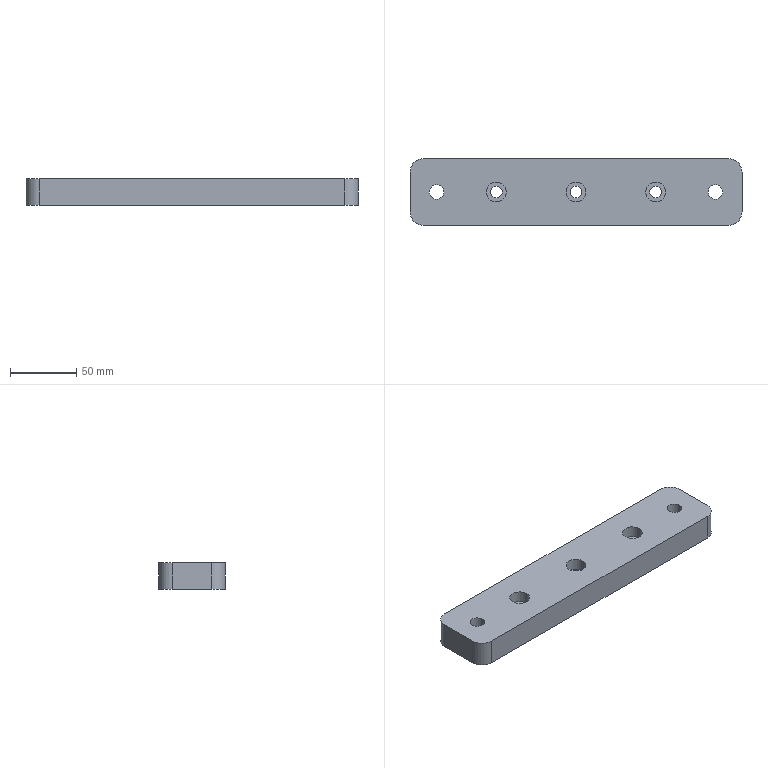Part | SolidWorks | features 3DProfileFeature 2, HoleWzd 2, Extrusion 1, Fillet 1, LPattern 1 | 1 solid | 39 faces | box 250 x 50 x 20 mm | volume 234104 mm3 | cylinder 24 | plane 11 | cone 4 | commonest cylinder face diameters 9 x6 15 x6 11 x4 18 x4 20 x4
STEP:
#1=CARTESIAN_POINT('',(64.,0.,0.025));
#2=VERTEX_POINT('',#1);
#3=CARTESIAN_POINT('',(46.,0.,0.025));
#4=VERTEX_POINT('',#3);
#5=CARTESIAN_POINT('',(55.,0.,0.025));
#6=DIRECTION('',(0.,0.,-1.));
#7=DIRECTION('',(-1.,0.,0.));
#8=AXIS2_PLACEMENT_3D('',#5,#6,#7);
#9=CIRCLE('',#8,9.);
#10=EDGE_CURVE('',#2,#4,#9,.T.);
#11=ORIENTED_EDGE('',*,*,#10,.F.);
#12=CARTESIAN_POINT('',(64.025,0.,0.));
#13=VERTEX_POINT('',#12);
#14=CARTESIAN_POINT('',(64.025,0.,0.));
#15=DIRECTION('',(0.7071,0.,-0.7071));
#16=VECTOR('',#15,1000.);
#17=LINE('',#14,#16);
#18=EDGE_CURVE('',#2,#13,#17,.T.);
#19=ORIENTED_EDGE('',*,*,#18,.T.);
#20=CARTESIAN_POINT('',(45.975,0.,0.));
#21=VERTEX_POINT('',#20);
#22=CARTESIAN_POINT('',(55.,0.,0.));
#23=DIRECTION('',(0.,0.,-1.));
#24=DIRECTION('',(-1.,0.,0.));
#25=AXIS2_PLACEMENT_3D('',#22,#23,#24);
#26=CIRCLE('',#25,9.025);
#27=EDGE_CURVE('',#13,#21,#26,.T.);
#28=ORIENTED_EDGE('',*,*,#27,.T.);
#29=CARTESIAN_POINT('',(45.975,0.,0.));
#30=DIRECTION('',(-0.7071,0.,-0.7071));
#31=VECTOR('',#30,1000.);
#32=LINE('',#29,#31);
#33=EDGE_CURVE('',#4,#21,#32,.T.);
#34=ORIENTED_EDGE('',*,*,#33,.F.);
#35=EDGE_LOOP('',(#11,#19,#28,#34));
#36=FACE_OUTER_BOUND('',#35,.T.);
#37=CARTESIAN_POINT('',(55.,0.,0.));
#38=DIRECTION('',(0.,0.,-1.));
#39=DIRECTION('',(-1.,0.,0.));
#40=AXIS2_PLACEMENT_3D('',#37,#38,#39);
#41=CONICAL_SURFACE('',#40,9.025,0.7854);
#42=ADVANCED_FACE('',(#36),#41,.F.);
#43=CARTESIAN_POINT('',(64.,0.,11.));
#44=VERTEX_POINT('',#43);
#45=CARTESIAN_POINT('',(46.,0.,11.));
#46=VERTEX_POINT('',#45);
#47=CARTESIAN_POINT('',(55.,0.,11.));
#48=DIRECTION('',(0.,0.,-1.));
#49=DIRECTION('',(-1.,0.,0.));
#50=AXIS2_PLACEMENT_3D('',#47,#48,#49);
#51=CIRCLE('',#50,9.);
#52=EDGE_CURVE('',#44,#46,#51,.T.);
#53=ORIENTED_EDGE('',*,*,#52,.F.);
#54=CARTESIAN_POINT('',(64.,0.,0.));
#55=DIRECTION('',(0.,0.,-1.));
#56=VECTOR('',#55,1000.);
#57=LINE('',#54,#56);
#58=EDGE_CURVE('',#44,#2,#57,.T.);
#59=ORIENTED_EDGE('',*,*,#58,.T.);
#60=ORIENTED_EDGE('',*,*,#10,.T.);
#61=CARTESIAN_POINT('',(46.,0.,0.));
#62=DIRECTION('',(0.,0.,-1.));
#63=VECTOR('',#62,1000.);
#64=LINE('',#61,#63);
#65=EDGE_CURVE('',#46,#4,#64,.T.);
#66=ORIENTED_EDGE('',*,*,#65,.F.);
#67=EDGE_LOOP('',(#53,#59,#60,#66));
#68=FACE_OUTER_BOUND('',#67,.T.);
#69=CARTESIAN_POINT('',(55.,0.,0.));
#70=DIRECTION('',(0.,0.,-1.));
#71=DIRECTION('',(-1.,0.,0.));
#72=AXIS2_PLACEMENT_3D('',#69,#70,#71);
#73=CYLINDRICAL_SURFACE('',#72,9.);
#74=ADVANCED_FACE('',(#68),#73,.F.);
#75=CARTESIAN_POINT('',(49.5,0.,20.));
#76=VERTEX_POINT('',#75);
#77=CARTESIAN_POINT('',(60.5,0.,20.));
#78=VERTEX_POINT('',#77);
#79=CARTESIAN_POINT('',(55.,0.,20.));
#80=DIRECTION('',(0.,0.,1.));
#81=DIRECTION('',(1.,0.,0.));
#82=AXIS2_PLACEMENT_3D('',#79,#80,#81);
#83=CIRCLE('',#82,5.5);
#84=EDGE_CURVE('',#76,#78,#83,.T.);
#85=ORIENTED_EDGE('',*,*,#84,.T.);
#86=CARTESIAN_POINT('',(60.5,0.,11.));
#87=VERTEX_POINT('',#86);
#88=CARTESIAN_POINT('',(60.5,0.,0.));
#89=DIRECTION('',(0.,0.,-1.));
#90=VECTOR('',#89,1000.);
#91=LINE('',#88,#90);
#92=EDGE_CURVE('',#78,#87,#91,.T.);
#93=ORIENTED_EDGE('',*,*,#92,.T.);
#94=CARTESIAN_POINT('',(49.5,0.,11.));
#95=VERTEX_POINT('',#94);
#96=CARTESIAN_POINT('',(55.,0.,11.));
#97=DIRECTION('',(0.,0.,-1.));
#98=DIRECTION('',(-1.,0.,0.));
#99=AXIS2_PLACEMENT_3D('',#96,#97,#98);
#100=CIRCLE('',#99,5.5);
#101=EDGE_CURVE('',#87,#95,#100,.T.);
#102=ORIENTED_EDGE('',*,*,#101,.T.);
#103=CARTESIAN_POINT('',(49.5,0.,0.));
#104=DIRECTION('',(0.,0.,-1.));
#105=VECTOR('',#104,1000.);
#106=LINE('',#103,#105);
#107=EDGE_CURVE('',#76,#95,#106,.T.);
#108=ORIENTED_EDGE('',*,*,#107,.F.);
#109=EDGE_LOOP('',(#85,#93,#102,#108));
#110=FACE_OUTER_BOUND('',#109,.T.);
#111=CARTESIAN_POINT('',(55.,0.,0.));
#112=DIRECTION('',(0.,0.,-1.));
#113=DIRECTION('',(-1.,0.,0.));
#114=AXIS2_PLACEMENT_3D('',#111,#112,#113);
#115=CYLINDRICAL_SURFACE('',#114,5.5);
#116=ADVANCED_FACE('',(#110),#115,.F.);
#117=CARTESIAN_POINT('',(-146.,0.,0.025));
#118=VERTEX_POINT('',#117);
#119=CARTESIAN_POINT('',(-164.,0.,0.025));
#120=VERTEX_POINT('',#119);
#121=CARTESIAN_POINT('',(-155.,0.,0.025));
#122=DIRECTION('',(0.,0.,-1.));
#123=DIRECTION('',(-1.,0.,0.));
#124=AXIS2_PLACEMENT_3D('',#121,#122,#123);
#125=CIRCLE('',#124,9.);
#126=EDGE_CURVE('',#118,#120,#125,.T.);
#127=ORIENTED_EDGE('',*,*,#126,.F.);
#128=CARTESIAN_POINT('',(-145.975,0.,0.));
#129=VERTEX_POINT('',#128);
#130=CARTESIAN_POINT('',(-145.975,0.,0.));
#131=DIRECTION('',(0.7071,0.,-0.7071));
#132=VECTOR('',#131,1000.);
#133=LINE('',#130,#132);
#134=EDGE_CURVE('',#118,#129,#133,.T.);
#135=ORIENTED_EDGE('',*,*,#134,.T.);
#136=CARTESIAN_POINT('',(-164.025,0.,0.));
#137=VERTEX_POINT('',#136);
#138=CARTESIAN_POINT('',(-155.,0.,0.));
#139=DIRECTION('',(0.,0.,-1.));
#140=DIRECTION('',(-1.,0.,0.));
#141=AXIS2_PLACEMENT_3D('',#138,#139,#140);
#142=CIRCLE('',#141,9.025);
#143=EDGE_CURVE('',#129,#137,#142,.T.);
#144=ORIENTED_EDGE('',*,*,#143,.T.);
#145=CARTESIAN_POINT('',(-164.025,0.,0.));
#146=DIRECTION('',(-0.7071,0.,-0.7071));
#147=VECTOR('',#146,1000.);
#148=LINE('',#145,#147);
#149=EDGE_CURVE('',#120,#137,#148,.T.);
#150=ORIENTED_EDGE('',*,*,#149,.F.);
#151=EDGE_LOOP('',(#127,#135,#144,#150));
#152=FACE_OUTER_BOUND('',#151,.T.);
#153=CARTESIAN_POINT('',(-155.,0.,0.));
#154=DIRECTION('',(0.,0.,-1.));
#155=DIRECTION('',(-1.,0.,0.));
#156=AXIS2_PLACEMENT_3D('',#153,#154,#155);
#157=CONICAL_SURFACE('',#156,9.025,0.7854);
#158=ADVANCED_FACE('',(#152),#157,.F.);
#159=CARTESIAN_POINT('',(-146.,0.,11.));
#160=VERTEX_POINT('',#159);
#161=CARTESIAN_POINT('',(-164.,0.,11.));
#162=VERTEX_POINT('',#161);
#163=CARTESIAN_POINT('',(-155.,0.,11.));
#164=DIRECTION('',(0.,0.,-1.));
#165=DIRECTION('',(-1.,0.,0.));
#166=AXIS2_PLACEMENT_3D('',#163,#164,#165);
#167=CIRCLE('',#166,9.);
#168=EDGE_CURVE('',#160,#162,#167,.T.);
#169=ORIENTED_EDGE('',*,*,#168,.F.);
#170=CARTESIAN_POINT('',(-146.,0.,0.));
#171=DIRECTION('',(0.,0.,-1.));
#172=VECTOR('',#171,1000.);
#173=LINE('',#170,#172);
#174=EDGE_CURVE('',#160,#118,#173,.T.);
#175=ORIENTED_EDGE('',*,*,#174,.T.);
#176=ORIENTED_EDGE('',*,*,#126,.T.);
#177=CARTESIAN_POINT('',(-164.,0.,0.));
#178=DIRECTION('',(0.,0.,-1.));
#179=VECTOR('',#178,1000.);
#180=LINE('',#177,#179);
#181=EDGE_CURVE('',#162,#120,#180,.T.);
#182=ORIENTED_EDGE('',*,*,#181,.F.);
#183=EDGE_LOOP('',(#169,#175,#176,#182));
#184=FACE_OUTER_BOUND('',#183,.T.);
#185=CARTESIAN_POINT('',(-155.,0.,0.));
#186=DIRECTION('',(0.,0.,-1.));
#187=DIRECTION('',(-1.,0.,0.));
#188=AXIS2_PLACEMENT_3D('',#185,#186,#187);
#189=CYLINDRICAL_SURFACE('',#188,9.);
#190=ADVANCED_FACE('',(#184),#189,.F.);
#191=CARTESIAN_POINT('',(-160.5,0.,20.));
#192=VERTEX_POINT('',#191);
#193=CARTESIAN_POINT('',(-149.5,0.,20.));
#194=VERTEX_POINT('',#193);
#195=CARTESIAN_POINT('',(-155.,0.,20.));
#196=DIRECTION('',(0.,0.,1.));
#197=DIRECTION('',(1.,0.,0.));
#198=AXIS2_PLACEMENT_3D('',#195,#196,#197);
#199=CIRCLE('',#198,5.5);
#200=EDGE_CURVE('',#192,#194,#199,.T.);
#201=ORIENTED_EDGE('',*,*,#200,.T.);
#202=CARTESIAN_POINT('',(-149.5,0.,11.));
#203=VERTEX_POINT('',#202);
#204=CARTESIAN_POINT('',(-149.5,0.,0.));
#205=DIRECTION('',(0.,0.,-1.));
#206=VECTOR('',#205,1000.);
#207=LINE('',#204,#206);
#208=EDGE_CURVE('',#194,#203,#207,.T.);
#209=ORIENTED_EDGE('',*,*,#208,.T.);
#210=CARTESIAN_POINT('',(-160.5,0.,11.));
#211=VERTEX_POINT('',#210);
#212=CARTESIAN_POINT('',(-155.,0.,11.));
#213=DIRECTION('',(0.,0.,-1.));
#214=DIRECTION('',(-1.,0.,0.));
#215=AXIS2_PLACEMENT_3D('',#212,#213,#214);
#216=CIRCLE('',#215,5.5);
#217=EDGE_CURVE('',#203,#211,#216,.T.);
#218=ORIENTED_EDGE('',*,*,#217,.T.);
#219=CARTESIAN_POINT('',(-160.5,0.,0.));
#220=DIRECTION('',(0.,0.,-1.));
#221=VECTOR('',#220,1000.);
#222=LINE('',#219,#221);
#223=EDGE_CURVE('',#192,#211,#222,.T.);
#224=ORIENTED_EDGE('',*,*,#223,.F.);
#225=EDGE_LOOP('',(#201,#209,#218,#224));
#226=FACE_OUTER_BOUND('',#225,.T.);
#227=CARTESIAN_POINT('',(-155.,0.,0.));
#228=DIRECTION('',(0.,0.,-1.));
#229=DIRECTION('',(-1.,0.,0.));
#230=AXIS2_PLACEMENT_3D('',#227,#228,#229);
#231=CYLINDRICAL_SURFACE('',#230,5.5);
#232=ADVANCED_FACE('',(#226),#231,.F.);
#233=CARTESIAN_POINT('',(-117.5,0.,11.));
#234=VERTEX_POINT('',#233);
#235=CARTESIAN_POINT('',(-102.5,0.,11.));
#236=VERTEX_POINT('',#235);
#237=CARTESIAN_POINT('',(-110.,0.,11.));
#238=DIRECTION('',(0.,0.,1.));
#239=DIRECTION('',(1.,0.,0.));
#240=AXIS2_PLACEMENT_3D('',#237,#238,#239);
#241=CIRCLE('',#240,7.5);
#242=EDGE_CURVE('',#234,#236,#241,.T.);
#243=ORIENTED_EDGE('',*,*,#242,.F.);
#244=CARTESIAN_POINT('',(-117.5,0.,20.));
#245=VERTEX_POINT('',#244);
#246=CARTESIAN_POINT('',(-117.5,0.,20.));
#247=DIRECTION('',(0.,0.,1.));
#248=VECTOR('',#247,1000.);
#249=LINE('',#246,#248);
#250=EDGE_CURVE('',#234,#245,#249,.T.);
#251=ORIENTED_EDGE('',*,*,#250,.T.);
#252=CARTESIAN_POINT('',(-102.5,0.,20.));
#253=VERTEX_POINT('',#252);
#254=CARTESIAN_POINT('',(-110.,0.,20.));
#255=DIRECTION('',(0.,0.,1.));
#256=DIRECTION('',(1.,0.,0.));
#257=AXIS2_PLACEMENT_3D('',#254,#255,#256);
#258=CIRCLE('',#257,7.5);
#259=EDGE_CURVE('',#245,#253,#258,.T.);
#260=ORIENTED_EDGE('',*,*,#259,.T.);
#261=CARTESIAN_POINT('',(-102.5,0.,20.));
#262=DIRECTION('',(0.,0.,1.));
#263=VECTOR('',#262,1000.);
#264=LINE('',#261,#263);
#265=EDGE_CURVE('',#236,#253,#264,.T.);
#266=ORIENTED_EDGE('',*,*,#265,.F.);
#267=EDGE_LOOP('',(#243,#251,#260,#266));
#268=FACE_OUTER_BOUND('',#267,.T.);
#269=CARTESIAN_POINT('',(-110.,0.,20.));
#270=DIRECTION('',(0.,0.,1.));
#271=DIRECTION('',(1.,0.,0.));
#272=AXIS2_PLACEMENT_3D('',#269,#270,#271);
#273=CYLINDRICAL_SURFACE('',#272,7.5);
#274=ADVANCED_FACE('',(#268),#273,.F.);
#275=CARTESIAN_POINT('',(-114.5,0.,0.));
#276=VERTEX_POINT('',#275);
#277=CARTESIAN_POINT('',(-105.5,0.,0.));
#278=VERTEX_POINT('',#277);
#279=CARTESIAN_POINT('',(-110.,0.,0.));
#280=DIRECTION('',(0.,0.,1.));
#281=DIRECTION('',(1.,0.,0.));
#282=AXIS2_PLACEMENT_3D('',#279,#280,#281);
#283=CIRCLE('',#282,4.5);
#284=EDGE_CURVE('',#276,#278,#283,.T.);
#285=ORIENTED_EDGE('',*,*,#284,.F.);
#286=CARTESIAN_POINT('',(-114.5,0.,11.));
#287=VERTEX_POINT('',#286);
#288=CARTESIAN_POINT('',(-114.5,0.,20.));
#289=DIRECTION('',(0.,0.,1.));
#290=VECTOR('',#289,1000.);
#291=LINE('',#288,#290);
#292=EDGE_CURVE('',#276,#287,#291,.T.);
#293=ORIENTED_EDGE('',*,*,#292,.T.);
#294=CARTESIAN_POINT('',(-105.5,0.,11.));
#295=VERTEX_POINT('',#294);
#296=CARTESIAN_POINT('',(-110.,0.,11.));
#297=DIRECTION('',(0.,0.,1.));
#298=DIRECTION('',(1.,0.,0.));
#299=AXIS2_PLACEMENT_3D('',#296,#297,#298);
#300=CIRCLE('',#299,4.5);
#301=EDGE_CURVE('',#287,#295,#300,.T.);
#302=ORIENTED_EDGE('',*,*,#301,.T.);
#303=CARTESIAN_POINT('',(-105.5,0.,20.));
#304=DIRECTION('',(0.,0.,1.));
#305=VECTOR('',#304,1000.);
#306=LINE('',#303,#305);
#307=EDGE_CURVE('',#278,#295,#306,.T.);
#308=ORIENTED_EDGE('',*,*,#307,.F.);
#309=EDGE_LOOP('',(#285,#293,#302,#308));
#310=FACE_OUTER_BOUND('',#309,.T.);
#311=CARTESIAN_POINT('',(-110.,0.,20.));
#312=DIRECTION('',(0.,0.,1.));
#313=DIRECTION('',(1.,0.,0.));
#314=AXIS2_PLACEMENT_3D('',#311,#312,#313);
#315=CYLINDRICAL_SURFACE('',#314,4.5);
#316=ADVANCED_FACE('',(#310),#315,.F.);
#317=CARTESIAN_POINT('',(-57.5,0.,11.));
#318=VERTEX_POINT('',#317);
#319=CARTESIAN_POINT('',(-42.5,0.,11.));
#320=VERTEX_POINT('',#319);
#321=CARTESIAN_POINT('',(-50.,0.,11.));
#322=DIRECTION('',(0.,0.,1.));
#323=DIRECTION('',(1.,0.,0.));
#324=AXIS2_PLACEMENT_3D('',#321,#322,#323);
#325=CIRCLE('',#324,7.5);
#326=EDGE_CURVE('',#318,#320,#325,.T.);
#327=ORIENTED_EDGE('',*,*,#326,.F.);
#328=CARTESIAN_POINT('',(-57.5,0.,20.));
#329=VERTEX_POINT('',#328);
#330=CARTESIAN_POINT('',(-57.5,0.,20.));
#331=DIRECTION('',(0.,0.,1.));
#332=VECTOR('',#331,1000.);
#333=LINE('',#330,#332);
#334=EDGE_CURVE('',#318,#329,#333,.T.);
#335=ORIENTED_EDGE('',*,*,#334,.T.);
#336=CARTESIAN_POINT('',(-42.5,0.,20.));
#337=VERTEX_POINT('',#336);
#338=CARTESIAN_POINT('',(-50.,0.,20.));
#339=DIRECTION('',(0.,0.,1.));
#340=DIRECTION('',(1.,0.,0.));
#341=AXIS2_PLACEMENT_3D('',#338,#339,#340);
#342=CIRCLE('',#341,7.5);
#343=EDGE_CURVE('',#329,#337,#342,.T.);
#344=ORIENTED_EDGE('',*,*,#343,.T.);
#345=CARTESIAN_POINT('',(-42.5,0.,20.));
#346=DIRECTION('',(0.,0.,1.));
#347=VECTOR('',#346,1000.);
#348=LINE('',#345,#347);
#349=EDGE_CURVE('',#320,#337,#348,.T.);
#350=ORIENTED_EDGE('',*,*,#349,.F.);
#351=EDGE_LOOP('',(#327,#335,#344,#350));
#352=FACE_OUTER_BOUND('',#351,.T.);
#353=CARTESIAN_POINT('',(-50.,0.,20.));
#354=DIRECTION('',(0.,0.,1.));
#355=DIRECTION('',(1.,0.,0.));
#356=AXIS2_PLACEMENT_3D('',#353,#354,#355);
#357=CYLINDRICAL_SURFACE('',#356,7.5);
#358=ADVANCED_FACE('',(#352),#357,.F.);
#359=CARTESIAN_POINT('',(-54.5,0.,0.));
#360=VERTEX_POINT('',#359);
#361=CARTESIAN_POINT('',(-45.5,0.,0.));
#362=VERTEX_POINT('',#361);
#363=CARTESIAN_POINT('',(-50.,0.,0.));
#364=DIRECTION('',(0.,0.,1.));
#365=DIRECTION('',(1.,0.,0.));
#366=AXIS2_PLACEMENT_3D('',#363,#364,#365);
#367=CIRCLE('',#366,4.5);
#368=EDGE_CURVE('',#360,#362,#367,.T.);
#369=ORIENTED_EDGE('',*,*,#368,.F.);
#370=CARTESIAN_POINT('',(-54.5,0.,11.));
#371=VERTEX_POINT('',#370);
#372=CARTESIAN_POINT('',(-54.5,0.,20.));
#373=DIRECTION('',(0.,0.,1.));
#374=VECTOR('',#373,1000.);
#375=LINE('',#372,#374);
#376=EDGE_CURVE('',#360,#371,#375,.T.);
#377=ORIENTED_EDGE('',*,*,#376,.T.);
#378=CARTESIAN_POINT('',(-45.5,0.,11.));
#379=VERTEX_POINT('',#378);
#380=CARTESIAN_POINT('',(-50.,0.,11.));
#381=DIRECTION('',(0.,0.,1.));
#382=DIRECTION('',(1.,0.,0.));
#383=AXIS2_PLACEMENT_3D('',#380,#381,#382);
#384=CIRCLE('',#383,4.5);
#385=EDGE_CURVE('',#371,#379,#384,.T.);
#386=ORIENTED_EDGE('',*,*,#385,.T.);
#387=CARTESIAN_POINT('',(-45.5,0.,20.));
#388=DIRECTION('',(0.,0.,1.));
#389=VECTOR('',#388,1000.);
#390=LINE('',#387,#389);
#391=EDGE_CURVE('',#362,#379,#390,.T.);
#392=ORIENTED_EDGE('',*,*,#391,.F.);
#393=EDGE_LOOP('',(#369,#377,#386,#392));
#394=FACE_OUTER_BOUND('',#393,.T.);
#395=CARTESIAN_POINT('',(-50.,0.,20.));
#396=DIRECTION('',(0.,0.,1.));
#397=DIRECTION('',(1.,0.,0.));
#398=AXIS2_PLACEMENT_3D('',#395,#396,#397);
#399=CYLINDRICAL_SURFACE('',#398,4.5);
#400=ADVANCED_FACE('',(#394),#399,.F.);
#401=CARTESIAN_POINT('',(2.5,0.,11.));
#402=VERTEX_POINT('',#401);
#403=CARTESIAN_POINT('',(17.5,0.,11.));
#404=VERTEX_POINT('',#403);
#405=CARTESIAN_POINT('',(10.,0.,11.));
#406=DIRECTION('',(0.,0.,1.));
#407=DIRECTION('',(1.,0.,0.));
#408=AXIS2_PLACEMENT_3D('',#405,#406,#407);
#409=CIRCLE('',#408,7.5);
#410=EDGE_CURVE('',#402,#404,#409,.T.);
#411=ORIENTED_EDGE('',*,*,#410,.F.);
#412=CARTESIAN_POINT('',(2.5,0.,20.));
#413=VERTEX_POINT('',#412);
#414=CARTESIAN_POINT('',(2.5,0.,20.));
#415=DIRECTION('',(0.,0.,1.));
#416=VECTOR('',#415,1000.);
#417=LINE('',#414,#416);
#418=EDGE_CURVE('',#402,#413,#417,.T.);
#419=ORIENTED_EDGE('',*,*,#418,.T.);
#420=CARTESIAN_POINT('',(17.5,0.,20.));
#421=VERTEX_POINT('',#420);
#422=CARTESIAN_POINT('',(10.,0.,20.));
#423=DIRECTION('',(0.,0.,1.));
#424=DIRECTION('',(1.,0.,0.));
#425=AXIS2_PLACEMENT_3D('',#422,#423,#424);
#426=CIRCLE('',#425,7.5);
#427=EDGE_CURVE('',#413,#421,#426,.T.);
#428=ORIENTED_EDGE('',*,*,#427,.T.);
#429=CARTESIAN_POINT('',(17.5,0.,20.));
#430=DIRECTION('',(0.,0.,1.));
#431=VECTOR('',#430,1000.);
#432=LINE('',#429,#431);
#433=EDGE_CURVE('',#404,#421,#432,.T.);
#434=ORIENTED_EDGE('',*,*,#433,.F.);
#435=EDGE_LOOP('',(#411,#419,#428,#434));
#436=FACE_OUTER_BOUND('',#435,.T.);
#437=CARTESIAN_POINT('',(10.,0.,20.));
#438=DIRECTION('',(0.,0.,1.));
#439=DIRECTION('',(1.,0.,0.));
#440=AXIS2_PLACEMENT_3D('',#437,#438,#439);
#441=CYLINDRICAL_SURFACE('',#440,7.5);
#442=ADVANCED_FACE('',(#436),#441,.F.);
#443=CARTESIAN_POINT('',(5.5,0.,0.));
#444=VERTEX_POINT('',#443);
#445=CARTESIAN_POINT('',(14.5,0.,0.));
#446=VERTEX_POINT('',#445);
#447=CARTESIAN_POINT('',(10.,0.,0.));
#448=DIRECTION('',(0.,0.,1.));
#449=DIRECTION('',(1.,0.,0.));
#450=AXIS2_PLACEMENT_3D('',#447,#448,#449);
#451=CIRCLE('',#450,4.5);
#452=EDGE_CURVE('',#444,#446,#451,.T.);
#453=ORIENTED_EDGE('',*,*,#452,.F.);
#454=CARTESIAN_POINT('',(5.5,0.,11.));
#455=VERTEX_POINT('',#454);
#456=CARTESIAN_POINT('',(5.5,0.,20.));
#457=DIRECTION('',(0.,0.,1.));
#458=VECTOR('',#457,1000.);
#459=LINE('',#456,#458);
#460=EDGE_CURVE('',#444,#455,#459,.T.);
#461=ORIENTED_EDGE('',*,*,#460,.T.);
#462=CARTESIAN_POINT('',(14.5,0.,11.));
#463=VERTEX_POINT('',#462);
#464=CARTESIAN_POINT('',(10.,0.,11.));
#465=DIRECTION('',(0.,0.,1.));
#466=DIRECTION('',(1.,0.,0.));
#467=AXIS2_PLACEMENT_3D('',#464,#465,#466);
#468=CIRCLE('',#467,4.5);
#469=EDGE_CURVE('',#455,#463,#468,.T.);
#470=ORIENTED_EDGE('',*,*,#469,.T.);
#471=CARTESIAN_POINT('',(14.5,0.,20.));
#472=DIRECTION('',(0.,0.,1.));
#473=VECTOR('',#472,1000.);
#474=LINE('',#471,#473);
#475=EDGE_CURVE('',#446,#463,#474,.T.);
#476=ORIENTED_EDGE('',*,*,#475,.F.);
#477=EDGE_LOOP('',(#453,#461,#470,#476));
#478=FACE_OUTER_BOUND('',#477,.T.);
#479=CARTESIAN_POINT('',(10.,0.,20.));
#480=DIRECTION('',(0.,0.,1.));
#481=DIRECTION('',(1.,0.,0.));
#482=AXIS2_PLACEMENT_3D('',#479,#480,#481);
#483=CYLINDRICAL_SURFACE('',#482,4.5);
#484=ADVANCED_FACE('',(#478),#483,.F.);
#485=CARTESIAN_POINT('',(-175.,15.,0.));
#486=VERTEX_POINT('',#485);
#487=CARTESIAN_POINT('',(-175.,-15.,0.));
#488=VERTEX_POINT('',#487);
#489=CARTESIAN_POINT('',(-175.,-25.,0.));
#490=DIRECTION('',(0.,-1.,0.));
#491=VECTOR('',#490,1000.);
#492=LINE('',#489,#491);
#493=EDGE_CURVE('',#486,#488,#492,.T.);
#494=ORIENTED_EDGE('',*,*,#493,.T.);
#495=CARTESIAN_POINT('',(-175.,-15.,20.));
#496=VERTEX_POINT('',#495);
#497=CARTESIAN_POINT('',(-175.,-15.,20.));
#498=DIRECTION('',(0.,0.,1.));
#499=VECTOR('',#498,1000.);
#500=LINE('',#497,#499);
#501=EDGE_CURVE('',#488,#496,#500,.T.);
#502=ORIENTED_EDGE('',*,*,#501,.T.);
#503=CARTESIAN_POINT('',(-175.,15.,20.));
#504=VERTEX_POINT('',#503);
#505=CARTESIAN_POINT('',(-175.,-25.,20.));
#506=DIRECTION('',(0.,-1.,0.));
#507=VECTOR('',#506,1000.);
#508=LINE('',#505,#507);
#509=EDGE_CURVE('',#504,#496,#508,.T.);
#510=ORIENTED_EDGE('',*,*,#509,.F.);
#511=CARTESIAN_POINT('',(-175.,15.,20.));
#512=DIRECTION('',(0.,0.,-1.));
#513=VECTOR('',#512,1000.);
#514=LINE('',#511,#513);
#515=EDGE_CURVE('',#504,#486,#514,.T.);
#516=ORIENTED_EDGE('',*,*,#515,.T.);
#517=EDGE_LOOP('',(#494,#502,#510,#516));
#518=FACE_OUTER_BOUND('',#517,.T.);
#519=CARTESIAN_POINT('',(-175.,-25.,20.));
#520=DIRECTION('',(1.,0.,0.));
#521=DIRECTION('',(0.,0.,-1.));
#522=AXIS2_PLACEMENT_3D('',#519,#520,#521);
#523=PLANE('',#522);
#524=ADVANCED_FACE('',(#518),#523,.F.);
#525=CARTESIAN_POINT('',(-165.,-25.,0.));
#526=VERTEX_POINT('',#525);
#527=CARTESIAN_POINT('',(65.,-25.,0.));
#528=VERTEX_POINT('',#527);
#529=CARTESIAN_POINT('',(75.,-25.,0.));
#530=DIRECTION('',(1.,0.,0.));
#531=VECTOR('',#530,1000.);
#532=LINE('',#529,#531);
#533=EDGE_CURVE('',#526,#528,#532,.T.);
#534=ORIENTED_EDGE('',*,*,#533,.T.);
#535=CARTESIAN_POINT('',(65.,-25.,20.));
#536=VERTEX_POINT('',#535);
#537=CARTESIAN_POINT('',(65.,-25.,20.));
#538=DIRECTION('',(0.,0.,1.));
#539=VECTOR('',#538,1000.);
#540=LINE('',#537,#539);
#541=EDGE_CURVE('',#528,#536,#540,.T.);
#542=ORIENTED_EDGE('',*,*,#541,.T.);
#543=CARTESIAN_POINT('',(-165.,-25.,20.));
#544=VERTEX_POINT('',#543);
#545=CARTESIAN_POINT('',(75.,-25.,20.));
#546=DIRECTION('',(1.,0.,0.));
#547=VECTOR('',#546,1000.);
#548=LINE('',#545,#547);
#549=EDGE_CURVE('',#544,#536,#548,.T.);
#550=ORIENTED_EDGE('',*,*,#549,.F.);
#551=CARTESIAN_POINT('',(-165.,-25.,20.));
#552=DIRECTION('',(0.,0.,-1.));
#553=VECTOR('',#552,1000.);
#554=LINE('',#551,#553);
#555=EDGE_CURVE('',#544,#526,#554,.T.);
#556=ORIENTED_EDGE('',*,*,#555,.T.);
#557=EDGE_LOOP('',(#534,#542,#550,#556));
#558=FACE_OUTER_BOUND('',#557,.T.);
#559=CARTESIAN_POINT('',(75.,-25.,20.));
#560=DIRECTION('',(0.,1.,0.));
#561=DIRECTION('',(-1.,0.,0.));
#562=AXIS2_PLACEMENT_3D('',#559,#560,#561);
#563=PLANE('',#562);
#564=ADVANCED_FACE('',(#558),#563,.F.);
#565=CARTESIAN_POINT('',(75.,-15.,20.));
#566=VERTEX_POINT('',#565);
#567=CARTESIAN_POINT('',(75.,15.,20.));
#568=VERTEX_POINT('',#567);
#569=CARTESIAN_POINT('',(75.,-25.,20.));
#570=DIRECTION('',(0.,1.,0.));
#571=VECTOR('',#570,1000.);
#572=LINE('',#569,#571);
#573=EDGE_CURVE('',#566,#568,#572,.T.);
#574=ORIENTED_EDGE('',*,*,#573,.F.);
#575=CARTESIAN_POINT('',(75.,-15.,0.));
#576=VERTEX_POINT('',#575);
#577=CARTESIAN_POINT('',(75.,-15.,20.));
#578=DIRECTION('',(0.,0.,-1.));
#579=VECTOR('',#578,1000.);
#580=LINE('',#577,#579);
#581=EDGE_CURVE('',#566,#576,#580,.T.);
#582=ORIENTED_EDGE('',*,*,#581,.T.);
#583=CARTESIAN_POINT('',(75.,15.,0.));
#584=VERTEX_POINT('',#583);
#585=CARTESIAN_POINT('',(75.,-25.,0.));
#586=DIRECTION('',(0.,1.,0.));
#587=VECTOR('',#586,1000.);
#588=LINE('',#585,#587);
#589=EDGE_CURVE('',#576,#584,#588,.T.);
#590=ORIENTED_EDGE('',*,*,#589,.T.);
#591=CARTESIAN_POINT('',(75.,15.,20.));
#592=DIRECTION('',(0.,0.,1.));
#593=VECTOR('',#592,1000.);
#594=LINE('',#591,#593);
#595=EDGE_CURVE('',#584,#568,#594,.T.);
#596=ORIENTED_EDGE('',*,*,#595,.T.);
#597=EDGE_LOOP('',(#574,#582,#590,#596));
#598=FACE_OUTER_BOUND('',#597,.T.);
#599=CARTESIAN_POINT('',(75.,-25.,20.));
#600=DIRECTION('',(-1.,0.,0.));
#601=DIRECTION('',(0.,0.,1.));
#602=AXIS2_PLACEMENT_3D('',#599,#600,#601);
#603=PLANE('',#602);
#604=ADVANCED_FACE('',(#598),#603,.F.);
#605=CARTESIAN_POINT('',(65.,25.,0.));
#606=VERTEX_POINT('',#605);
#607=CARTESIAN_POINT('',(-165.,25.,0.));
#608=VERTEX_POINT('',#607);
#609=CARTESIAN_POINT('',(75.,25.,0.));
#610=DIRECTION('',(-1.,0.,0.));
#611=VECTOR('',#610,1000.);
#612=LINE('',#609,#611);
#613=EDGE_CURVE('',#606,#608,#612,.T.);
#614=ORIENTED_EDGE('',*,*,#613,.T.);
#615=CARTESIAN_POINT('',(-165.,25.,20.));
#616=VERTEX_POINT('',#615);
#617=CARTESIAN_POINT('',(-165.,25.,20.));
#618=DIRECTION('',(0.,0.,1.));
#619=VECTOR('',#618,1000.);
#620=LINE('',#617,#619);
#621=EDGE_CURVE('',#608,#616,#620,.T.);
#622=ORIENTED_EDGE('',*,*,#621,.T.);
#623=CARTESIAN_POINT('',(65.,25.,20.));
#624=VERTEX_POINT('',#623);
#625=CARTESIAN_POINT('',(75.,25.,20.));
#626=DIRECTION('',(-1.,0.,0.));
#627=VECTOR('',#626,1000.);
#628=LINE('',#625,#627);
#629=EDGE_CURVE('',#624,#616,#628,.T.);
#630=ORIENTED_EDGE('',*,*,#629,.F.);
#631=CARTESIAN_POINT('',(65.,25.,20.));
#632=DIRECTION('',(0.,0.,-1.));
#633=VECTOR('',#632,1000.);
#634=LINE('',#631,#633);
#635=EDGE_CURVE('',#624,#606,#634,.T.);
#636=ORIENTED_EDGE('',*,*,#635,.T.);
#637=EDGE_LOOP('',(#614,#622,#630,#636));
#638=FACE_OUTER_BOUND('',#637,.T.);
#639=CARTESIAN_POINT('',(75.,25.,20.));
#640=DIRECTION('',(0.,-1.,0.));
#641=DIRECTION('',(1.,0.,0.));
#642=AXIS2_PLACEMENT_3D('',#639,#640,#641);
#643=PLANE('',#642);
#644=ADVANCED_FACE('',(#638),#643,.F.);
#645=ORIENTED_EDGE('',*,*,#84,.F.);
#646=CARTESIAN_POINT('',(55.,0.,20.));
#647=DIRECTION('',(0.,0.,1.));
#648=DIRECTION('',(1.,0.,0.));
#649=AXIS2_PLACEMENT_3D('',#646,#647,#648);
#650=CIRCLE('',#649,5.5);
#651=EDGE_CURVE('',#78,#76,#650,.T.);
#652=ORIENTED_EDGE('',*,*,#651,.F.);
#653=EDGE_LOOP('',(#645,#652));
#654=FACE_BOUND('',#653,.T.);
#655=ORIENTED_EDGE('',*,*,#200,.F.);
#656=CARTESIAN_POINT('',(-155.,0.,20.));
#657=DIRECTION('',(0.,0.,1.));
#658=DIRECTION('',(1.,0.,0.));
#659=AXIS2_PLACEMENT_3D('',#656,#657,#658);
#660=CIRCLE('',#659,5.5);
#661=EDGE_CURVE('',#194,#192,#660,.T.);
#662=ORIENTED_EDGE('',*,*,#661,.F.);
#663=EDGE_LOOP('',(#655,#662));
#664=FACE_BOUND('',#663,.T.);
#665=CARTESIAN_POINT('',(-110.,0.,20.));
#666=DIRECTION('',(0.,0.,1.));
#667=DIRECTION('',(1.,0.,0.));
#668=AXIS2_PLACEMENT_3D('',#665,#666,#667);
#669=CIRCLE('',#668,7.5);
#670=EDGE_CURVE('',#253,#245,#669,.T.);
#671=ORIENTED_EDGE('',*,*,#670,.F.);
#672=ORIENTED_EDGE('',*,*,#259,.F.);
#673=EDGE_LOOP('',(#671,#672));
#674=FACE_BOUND('',#673,.T.);
#675=CARTESIAN_POINT('',(-50.,0.,20.));
#676=DIRECTION('',(0.,0.,1.));
#677=DIRECTION('',(1.,0.,0.));
#678=AXIS2_PLACEMENT_3D('',#675,#676,#677);
#679=CIRCLE('',#678,7.5);
#680=EDGE_CURVE('',#337,#329,#679,.T.);
#681=ORIENTED_EDGE('',*,*,#680,.F.);
#682=ORIENTED_EDGE('',*,*,#343,.F.);
#683=EDGE_LOOP('',(#681,#682));
#684=FACE_BOUND('',#683,.T.);
#685=CARTESIAN_POINT('',(10.,0.,20.));
#686=DIRECTION('',(0.,0.,1.));
#687=DIRECTION('',(1.,0.,0.));
#688=AXIS2_PLACEMENT_3D('',#685,#686,#687);
#689=CIRCLE('',#688,7.5);
#690=EDGE_CURVE('',#421,#413,#689,.T.);
#691=ORIENTED_EDGE('',*,*,#690,.F.);
#692=ORIENTED_EDGE('',*,*,#427,.F.);
#693=EDGE_LOOP('',(#691,#692));
#694=FACE_BOUND('',#693,.T.);
#695=ORIENTED_EDGE('',*,*,#549,.T.);
#696=CARTESIAN_POINT('',(65.,-15.,20.));
#697=DIRECTION('',(0.,0.,1.));
#698=DIRECTION('',(1.,0.,0.));
#699=AXIS2_PLACEMENT_3D('',#696,#697,#698);
#700=CIRCLE('',#699,10.);
#701=EDGE_CURVE('',#536,#566,#700,.T.);
#702=ORIENTED_EDGE('',*,*,#701,.T.);
#703=ORIENTED_EDGE('',*,*,#573,.T.);
#704=CARTESIAN_POINT('',(65.,15.,20.));
#705=DIRECTION('',(0.,0.,1.));
#706=DIRECTION('',(1.,0.,0.));
#707=AXIS2_PLACEMENT_3D('',#704,#705,#706);
#708=CIRCLE('',#707,10.);
#709=EDGE_CURVE('',#568,#624,#708,.T.);
#710=ORIENTED_EDGE('',*,*,#709,.T.);
#711=ORIENTED_EDGE('',*,*,#629,.T.);
#712=CARTESIAN_POINT('',(-165.,15.,20.));
#713=DIRECTION('',(0.,0.,1.));
#714=DIRECTION('',(1.,0.,0.));
#715=AXIS2_PLACEMENT_3D('',#712,#713,#714);
#716=CIRCLE('',#715,10.);
#717=EDGE_CURVE('',#616,#504,#716,.T.);
#718=ORIENTED_EDGE('',*,*,#717,.T.);
#719=ORIENTED_EDGE('',*,*,#509,.T.);
#720=CARTESIAN_POINT('',(-165.,-15.,20.));
#721=DIRECTION('',(0.,0.,1.));
#722=DIRECTION('',(1.,0.,0.));
#723=AXIS2_PLACEMENT_3D('',#720,#721,#722);
#724=CIRCLE('',#723,10.);
#725=EDGE_CURVE('',#496,#544,#724,.T.);
#726=ORIENTED_EDGE('',*,*,#725,.T.);
#727=EDGE_LOOP('',(#695,#702,#703,#710,#711,#718,#719,#726));
#728=FACE_OUTER_BOUND('',#727,.T.);
#729=CARTESIAN_POINT('',(0.,0.,20.));
#730=DIRECTION('',(0.,0.,1.));
#731=DIRECTION('',(1.,0.,0.));
#732=AXIS2_PLACEMENT_3D('',#729,#730,#731);
#733=PLANE('',#732);
#734=ADVANCED_FACE('',(#654,#664,#674,#684,#694,#728),#733,.T.);
#735=CARTESIAN_POINT('',(55.,0.,0.));
#736=DIRECTION('',(0.,0.,-1.));
#737=DIRECTION('',(-1.,0.,0.));
#738=AXIS2_PLACEMENT_3D('',#735,#736,#737);
#739=CIRCLE('',#738,9.025);
#740=EDGE_CURVE('',#21,#13,#739,.T.);
#741=ORIENTED_EDGE('',*,*,#740,.F.);
#742=ORIENTED_EDGE('',*,*,#27,.F.);
#743=EDGE_LOOP('',(#741,#742));
#744=FACE_BOUND('',#743,.T.);
#745=CARTESIAN_POINT('',(-155.,0.,0.));
#746=DIRECTION('',(0.,0.,-1.));
#747=DIRECTION('',(-1.,0.,0.));
#748=AXIS2_PLACEMENT_3D('',#745,#746,#747);
#749=CIRCLE('',#748,9.025);
#750=EDGE_CURVE('',#137,#129,#749,.T.);
#751=ORIENTED_EDGE('',*,*,#750,.F.);
#752=ORIENTED_EDGE('',*,*,#143,.F.);
#753=EDGE_LOOP('',(#751,#752));
#754=FACE_BOUND('',#753,.T.);
#755=CARTESIAN_POINT('',(-110.,0.,0.));
#756=DIRECTION('',(0.,0.,1.));
#757=DIRECTION('',(1.,0.,0.));
#758=AXIS2_PLACEMENT_3D('',#755,#756,#757);
#759=CIRCLE('',#758,4.5);
#760=EDGE_CURVE('',#278,#276,#759,.T.);
#761=ORIENTED_EDGE('',*,*,#760,.T.);
#762=ORIENTED_EDGE('',*,*,#284,.T.);
#763=EDGE_LOOP('',(#761,#762));
#764=FACE_BOUND('',#763,.T.);
#765=CARTESIAN_POINT('',(-50.,0.,0.));
#766=DIRECTION('',(0.,0.,1.));
#767=DIRECTION('',(1.,0.,0.));
#768=AXIS2_PLACEMENT_3D('',#765,#766,#767);
#769=CIRCLE('',#768,4.5);
#770=EDGE_CURVE('',#362,#360,#769,.T.);
#771=ORIENTED_EDGE('',*,*,#770,.T.);
#772=ORIENTED_EDGE('',*,*,#368,.T.);
#773=EDGE_LOOP('',(#771,#772));
#774=FACE_BOUND('',#773,.T.);
#775=CARTESIAN_POINT('',(10.,0.,0.));
#776=DIRECTION('',(0.,0.,1.));
#777=DIRECTION('',(1.,0.,0.));
#778=AXIS2_PLACEMENT_3D('',#775,#776,#777);
#779=CIRCLE('',#778,4.5);
#780=EDGE_CURVE('',#446,#444,#779,.T.);
#781=ORIENTED_EDGE('',*,*,#780,.T.);
#782=ORIENTED_EDGE('',*,*,#452,.T.);
#783=EDGE_LOOP('',(#781,#782));
#784=FACE_BOUND('',#783,.T.);
#785=ORIENTED_EDGE('',*,*,#589,.F.);
#786=CARTESIAN_POINT('',(65.,-15.,0.));
#787=DIRECTION('',(0.,0.,-1.));
#788=DIRECTION('',(1.,0.,0.));
#789=AXIS2_PLACEMENT_3D('',#786,#787,#788);
#790=CIRCLE('',#789,10.);
#791=EDGE_CURVE('',#576,#528,#790,.T.);
#792=ORIENTED_EDGE('',*,*,#791,.T.);
#793=ORIENTED_EDGE('',*,*,#533,.F.);
#794=CARTESIAN_POINT('',(-165.,-15.,0.));
#795=DIRECTION('',(0.,0.,-1.));
#796=DIRECTION('',(1.,0.,0.));
#797=AXIS2_PLACEMENT_3D('',#794,#795,#796);
#798=CIRCLE('',#797,10.);
#799=EDGE_CURVE('',#526,#488,#798,.T.);
#800=ORIENTED_EDGE('',*,*,#799,.T.);
#801=ORIENTED_EDGE('',*,*,#493,.F.);
#802=CARTESIAN_POINT('',(-165.,15.,0.));
#803=DIRECTION('',(0.,0.,-1.));
#804=DIRECTION('',(1.,0.,0.));
#805=AXIS2_PLACEMENT_3D('',#802,#803,#804);
#806=CIRCLE('',#805,10.);
#807=EDGE_CURVE('',#486,#608,#806,.T.);
#808=ORIENTED_EDGE('',*,*,#807,.T.);
#809=ORIENTED_EDGE('',*,*,#613,.F.);
#810=CARTESIAN_POINT('',(65.,15.,0.));
#811=DIRECTION('',(0.,0.,-1.));
#812=DIRECTION('',(1.,0.,0.));
#813=AXIS2_PLACEMENT_3D('',#810,#811,#812);
#814=CIRCLE('',#813,10.);
#815=EDGE_CURVE('',#606,#584,#814,.T.);
#816=ORIENTED_EDGE('',*,*,#815,.T.);
#817=EDGE_LOOP('',(#785,#792,#793,#800,#801,#808,#809,#816));
#818=FACE_OUTER_BOUND('',#817,.T.);
#819=CARTESIAN_POINT('',(0.,0.,0.));
#820=DIRECTION('',(0.,0.,1.));
#821=DIRECTION('',(1.,0.,0.));
#822=AXIS2_PLACEMENT_3D('',#819,#820,#821);
#823=PLANE('',#822);
#824=ADVANCED_FACE('',(#744,#754,#764,#774,#784,#818),#823,.F.);
#825=ORIENTED_EDGE('',*,*,#701,.F.);
#826=ORIENTED_EDGE('',*,*,#541,.F.);
#827=ORIENTED_EDGE('',*,*,#791,.F.);
#828=ORIENTED_EDGE('',*,*,#581,.F.);
#829=EDGE_LOOP('',(#825,#826,#827,#828));
#830=FACE_OUTER_BOUND('',#829,.T.);
#831=CARTESIAN_POINT('',(65.,-15.,20.));
#832=DIRECTION('',(0.,0.,-1.));
#833=DIRECTION('',(-1.,0.,0.));
#834=AXIS2_PLACEMENT_3D('',#831,#832,#833);
#835=CYLINDRICAL_SURFACE('',#834,10.);
#836=ADVANCED_FACE('',(#830),#835,.T.);
#837=ORIENTED_EDGE('',*,*,#725,.F.);
#838=ORIENTED_EDGE('',*,*,#501,.F.);
#839=ORIENTED_EDGE('',*,*,#799,.F.);
#840=ORIENTED_EDGE('',*,*,#555,.F.);
#841=EDGE_LOOP('',(#837,#838,#839,#840));
#842=FACE_OUTER_BOUND('',#841,.T.);
#843=CARTESIAN_POINT('',(-165.,-15.,20.));
#844=DIRECTION('',(0.,0.,-1.));
#845=DIRECTION('',(-1.,0.,0.));
#846=AXIS2_PLACEMENT_3D('',#843,#844,#845);
#847=CYLINDRICAL_SURFACE('',#846,10.);
#848=ADVANCED_FACE('',(#842),#847,.T.);
#849=ORIENTED_EDGE('',*,*,#717,.F.);
#850=ORIENTED_EDGE('',*,*,#621,.F.);
#851=ORIENTED_EDGE('',*,*,#807,.F.);
#852=ORIENTED_EDGE('',*,*,#515,.F.);
#853=EDGE_LOOP('',(#849,#850,#851,#852));
#854=FACE_OUTER_BOUND('',#853,.T.);
#855=CARTESIAN_POINT('',(-165.,15.,20.));
#856=DIRECTION('',(0.,0.,-1.));
#857=DIRECTION('',(-1.,0.,0.));
#858=AXIS2_PLACEMENT_3D('',#855,#856,#857);
#859=CYLINDRICAL_SURFACE('',#858,10.);
#860=ADVANCED_FACE('',(#854),#859,.T.);
#861=ORIENTED_EDGE('',*,*,#709,.F.);
#862=ORIENTED_EDGE('',*,*,#595,.F.);
#863=ORIENTED_EDGE('',*,*,#815,.F.);
#864=ORIENTED_EDGE('',*,*,#635,.F.);
#865=EDGE_LOOP('',(#861,#862,#863,#864));
#866=FACE_OUTER_BOUND('',#865,.T.);
#867=CARTESIAN_POINT('',(65.,15.,20.));
#868=DIRECTION('',(0.,0.,-1.));
#869=DIRECTION('',(-1.,0.,0.));
#870=AXIS2_PLACEMENT_3D('',#867,#868,#869);
#871=CYLINDRICAL_SURFACE('',#870,10.);
#872=ADVANCED_FACE('',(#866),#871,.T.);
#873=ORIENTED_EDGE('',*,*,#460,.F.);
#874=ORIENTED_EDGE('',*,*,#780,.F.);
#875=ORIENTED_EDGE('',*,*,#475,.T.);
#876=CARTESIAN_POINT('',(10.,0.,11.));
#877=DIRECTION('',(0.,0.,1.));
#878=DIRECTION('',(1.,0.,0.));
#879=AXIS2_PLACEMENT_3D('',#876,#877,#878);
#880=CIRCLE('',#879,4.5);
#881=EDGE_CURVE('',#463,#455,#880,.T.);
#882=ORIENTED_EDGE('',*,*,#881,.T.);
#883=EDGE_LOOP('',(#873,#874,#875,#882));
#884=FACE_OUTER_BOUND('',#883,.T.);
#885=CARTESIAN_POINT('',(10.,0.,20.));
#886=DIRECTION('',(0.,0.,1.));
#887=DIRECTION('',(1.,0.,0.));
#888=AXIS2_PLACEMENT_3D('',#885,#886,#887);
#889=CYLINDRICAL_SURFACE('',#888,4.5);
#890=ADVANCED_FACE('',(#884),#889,.F.);
#891=ORIENTED_EDGE('',*,*,#881,.F.);
#892=ORIENTED_EDGE('',*,*,#469,.F.);
#893=EDGE_LOOP('',(#891,#892));
#894=FACE_BOUND('',#893,.T.);
#895=CARTESIAN_POINT('',(10.,0.,11.));
#896=DIRECTION('',(0.,0.,1.));
#897=DIRECTION('',(1.,0.,0.));
#898=AXIS2_PLACEMENT_3D('',#895,#896,#897);
#899=CIRCLE('',#898,7.5);
#900=EDGE_CURVE('',#404,#402,#899,.T.);
#901=ORIENTED_EDGE('',*,*,#900,.T.);
#902=ORIENTED_EDGE('',*,*,#410,.T.);
#903=EDGE_LOOP('',(#901,#902));
#904=FACE_OUTER_BOUND('',#903,.T.);
#905=CARTESIAN_POINT('',(14.5,0.,11.));
#906=DIRECTION('',(0.,0.,-1.));
#907=DIRECTION('',(-1.,0.,0.));
#908=AXIS2_PLACEMENT_3D('',#905,#906,#907);
#909=PLANE('',#908);
#910=ADVANCED_FACE('',(#894,#904),#909,.F.);
#911=ORIENTED_EDGE('',*,*,#418,.F.);
#912=ORIENTED_EDGE('',*,*,#900,.F.);
#913=ORIENTED_EDGE('',*,*,#433,.T.);
#914=ORIENTED_EDGE('',*,*,#690,.T.);
#915=EDGE_LOOP('',(#911,#912,#913,#914));
#916=FACE_OUTER_BOUND('',#915,.T.);
#917=CARTESIAN_POINT('',(10.,0.,20.));
#918=DIRECTION('',(0.,0.,1.));
#919=DIRECTION('',(1.,0.,0.));
#920=AXIS2_PLACEMENT_3D('',#917,#918,#919);
#921=CYLINDRICAL_SURFACE('',#920,7.5);
#922=ADVANCED_FACE('',(#916),#921,.F.);
#923=ORIENTED_EDGE('',*,*,#376,.F.);
#924=ORIENTED_EDGE('',*,*,#770,.F.);
#925=ORIENTED_EDGE('',*,*,#391,.T.);
#926=CARTESIAN_POINT('',(-50.,0.,11.));
#927=DIRECTION('',(0.,0.,1.));
#928=DIRECTION('',(1.,0.,0.));
#929=AXIS2_PLACEMENT_3D('',#926,#927,#928);
#930=CIRCLE('',#929,4.5);
#931=EDGE_CURVE('',#379,#371,#930,.T.);
#932=ORIENTED_EDGE('',*,*,#931,.T.);
#933=EDGE_LOOP('',(#923,#924,#925,#932));
#934=FACE_OUTER_BOUND('',#933,.T.);
#935=CARTESIAN_POINT('',(-50.,0.,20.));
#936=DIRECTION('',(0.,0.,1.));
#937=DIRECTION('',(1.,0.,0.));
#938=AXIS2_PLACEMENT_3D('',#935,#936,#937);
#939=CYLINDRICAL_SURFACE('',#938,4.5);
#940=ADVANCED_FACE('',(#934),#939,.F.);
#941=ORIENTED_EDGE('',*,*,#931,.F.);
#942=ORIENTED_EDGE('',*,*,#385,.F.);
#943=EDGE_LOOP('',(#941,#942));
#944=FACE_BOUND('',#943,.T.);
#945=CARTESIAN_POINT('',(-50.,0.,11.));
#946=DIRECTION('',(0.,0.,1.));
#947=DIRECTION('',(1.,0.,0.));
#948=AXIS2_PLACEMENT_3D('',#945,#946,#947);
#949=CIRCLE('',#948,7.5);
#950=EDGE_CURVE('',#320,#318,#949,.T.);
#951=ORIENTED_EDGE('',*,*,#950,.T.);
#952=ORIENTED_EDGE('',*,*,#326,.T.);
#953=EDGE_LOOP('',(#951,#952));
#954=FACE_OUTER_BOUND('',#953,.T.);
#955=CARTESIAN_POINT('',(-45.5,0.,11.));
#956=DIRECTION('',(0.,0.,-1.));
#957=DIRECTION('',(-1.,0.,0.));
#958=AXIS2_PLACEMENT_3D('',#955,#956,#957);
#959=PLANE('',#958);
#960=ADVANCED_FACE('',(#944,#954),#959,.F.);
#961=ORIENTED_EDGE('',*,*,#334,.F.);
#962=ORIENTED_EDGE('',*,*,#950,.F.);
#963=ORIENTED_EDGE('',*,*,#349,.T.);
#964=ORIENTED_EDGE('',*,*,#680,.T.);
#965=EDGE_LOOP('',(#961,#962,#963,#964));
#966=FACE_OUTER_BOUND('',#965,.T.);
#967=CARTESIAN_POINT('',(-50.,0.,20.));
#968=DIRECTION('',(0.,0.,1.));
#969=DIRECTION('',(1.,0.,0.));
#970=AXIS2_PLACEMENT_3D('',#967,#968,#969);
#971=CYLINDRICAL_SURFACE('',#970,7.5);
#972=ADVANCED_FACE('',(#966),#971,.F.);
#973=ORIENTED_EDGE('',*,*,#292,.F.);
#974=ORIENTED_EDGE('',*,*,#760,.F.);
#975=ORIENTED_EDGE('',*,*,#307,.T.);
#976=CARTESIAN_POINT('',(-110.,0.,11.));
#977=DIRECTION('',(0.,0.,1.));
#978=DIRECTION('',(1.,0.,0.));
#979=AXIS2_PLACEMENT_3D('',#976,#977,#978);
#980=CIRCLE('',#979,4.5);
#981=EDGE_CURVE('',#295,#287,#980,.T.);
#982=ORIENTED_EDGE('',*,*,#981,.T.);
#983=EDGE_LOOP('',(#973,#974,#975,#982));
#984=FACE_OUTER_BOUND('',#983,.T.);
#985=CARTESIAN_POINT('',(-110.,0.,20.));
#986=DIRECTION('',(0.,0.,1.));
#987=DIRECTION('',(1.,0.,0.));
#988=AXIS2_PLACEMENT_3D('',#985,#986,#987);
#989=CYLINDRICAL_SURFACE('',#988,4.5);
#990=ADVANCED_FACE('',(#984),#989,.F.);
#991=ORIENTED_EDGE('',*,*,#981,.F.);
#992=ORIENTED_EDGE('',*,*,#301,.F.);
#993=EDGE_LOOP('',(#991,#992));
#994=FACE_BOUND('',#993,.T.);
#995=CARTESIAN_POINT('',(-110.,0.,11.));
#996=DIRECTION('',(0.,0.,1.));
#997=DIRECTION('',(1.,0.,0.));
#998=AXIS2_PLACEMENT_3D('',#995,#996,#997);
#999=CIRCLE('',#998,7.5);
#1000=EDGE_CURVE('',#236,#234,#999,.T.);
#1001=ORIENTED_EDGE('',*,*,#1000,.T.);
#1002=ORIENTED_EDGE('',*,*,#242,.T.);
#1003=EDGE_LOOP('',(#1001,#1002));
#1004=FACE_OUTER_BOUND('',#1003,.T.);
#1005=CARTESIAN_POINT('',(-105.5,0.,11.));
#1006=DIRECTION('',(0.,0.,-1.));
#1007=DIRECTION('',(-1.,0.,0.));
#1008=AXIS2_PLACEMENT_3D('',#1005,#1006,#1007);
#1009=PLANE('',#1008);
#1010=ADVANCED_FACE('',(#994,#1004),#1009,.F.);
#1011=ORIENTED_EDGE('',*,*,#250,.F.);
#1012=ORIENTED_EDGE('',*,*,#1000,.F.);
#1013=ORIENTED_EDGE('',*,*,#265,.T.);
#1014=ORIENTED_EDGE('',*,*,#670,.T.);
#1015=EDGE_LOOP('',(#1011,#1012,#1013,#1014));
#1016=FACE_OUTER_BOUND('',#1015,.T.);
#1017=CARTESIAN_POINT('',(-110.,0.,20.));
#1018=DIRECTION('',(0.,0.,1.));
#1019=DIRECTION('',(1.,0.,0.));
#1020=AXIS2_PLACEMENT_3D('',#1017,#1018,#1019);
#1021=CYLINDRICAL_SURFACE('',#1020,7.5);
#1022=ADVANCED_FACE('',(#1016),#1021,.F.);
#1023=ORIENTED_EDGE('',*,*,#208,.F.);
#1024=ORIENTED_EDGE('',*,*,#661,.T.);
#1025=ORIENTED_EDGE('',*,*,#223,.T.);
#1026=CARTESIAN_POINT('',(-155.,0.,11.));
#1027=DIRECTION('',(0.,0.,-1.));
#1028=DIRECTION('',(-1.,0.,0.));
#1029=AXIS2_PLACEMENT_3D('',#1026,#1027,#1028);
#1030=CIRCLE('',#1029,5.5);
#1031=EDGE_CURVE('',#211,#203,#1030,.T.);
#1032=ORIENTED_EDGE('',*,*,#1031,.T.);
#1033=EDGE_LOOP('',(#1023,#1024,#1025,#1032));
#1034=FACE_OUTER_BOUND('',#1033,.T.);
#1035=CARTESIAN_POINT('',(-155.,0.,0.));
#1036=DIRECTION('',(0.,0.,-1.));
#1037=DIRECTION('',(-1.,0.,0.));
#1038=AXIS2_PLACEMENT_3D('',#1035,#1036,#1037);
#1039=CYLINDRICAL_SURFACE('',#1038,5.5);
#1040=ADVANCED_FACE('',(#1034),#1039,.F.);
#1041=ORIENTED_EDGE('',*,*,#1031,.F.);
#1042=ORIENTED_EDGE('',*,*,#217,.F.);
#1043=EDGE_LOOP('',(#1041,#1042));
#1044=FACE_BOUND('',#1043,.T.);
#1045=CARTESIAN_POINT('',(-155.,0.,11.));
#1046=DIRECTION('',(0.,0.,-1.));
#1047=DIRECTION('',(-1.,0.,0.));
#1048=AXIS2_PLACEMENT_3D('',#1045,#1046,#1047);
#1049=CIRCLE('',#1048,9.);
#1050=EDGE_CURVE('',#162,#160,#1049,.T.);
#1051=ORIENTED_EDGE('',*,*,#1050,.T.);
#1052=ORIENTED_EDGE('',*,*,#168,.T.);
#1053=EDGE_LOOP('',(#1051,#1052));
#1054=FACE_OUTER_BOUND('',#1053,.T.);
#1055=CARTESIAN_POINT('',(-149.5,0.,11.));
#1056=DIRECTION('',(0.,0.,1.));
#1057=DIRECTION('',(1.,0.,0.));
#1058=AXIS2_PLACEMENT_3D('',#1055,#1056,#1057);
#1059=PLANE('',#1058);
#1060=ADVANCED_FACE('',(#1044,#1054),#1059,.F.);
#1061=ORIENTED_EDGE('',*,*,#174,.F.);
#1062=ORIENTED_EDGE('',*,*,#1050,.F.);
#1063=ORIENTED_EDGE('',*,*,#181,.T.);
#1064=CARTESIAN_POINT('',(-155.,0.,0.025));
#1065=DIRECTION('',(0.,0.,-1.));
#1066=DIRECTION('',(-1.,0.,0.));
#1067=AXIS2_PLACEMENT_3D('',#1064,#1065,#1066);
#1068=CIRCLE('',#1067,9.);
#1069=EDGE_CURVE('',#120,#118,#1068,.T.);
#1070=ORIENTED_EDGE('',*,*,#1069,.T.);
#1071=EDGE_LOOP('',(#1061,#1062,#1063,#1070));
#1072=FACE_OUTER_BOUND('',#1071,.T.);
#1073=CARTESIAN_POINT('',(-155.,0.,0.));
#1074=DIRECTION('',(0.,0.,-1.));
#1075=DIRECTION('',(-1.,0.,0.));
#1076=AXIS2_PLACEMENT_3D('',#1073,#1074,#1075);
#1077=CYLINDRICAL_SURFACE('',#1076,9.);
#1078=ADVANCED_FACE('',(#1072),#1077,.F.);
#1079=ORIENTED_EDGE('',*,*,#134,.F.);
#1080=ORIENTED_EDGE('',*,*,#1069,.F.);
#1081=ORIENTED_EDGE('',*,*,#149,.T.);
#1082=ORIENTED_EDGE('',*,*,#750,.T.);
#1083=EDGE_LOOP('',(#1079,#1080,#1081,#1082));
#1084=FACE_OUTER_BOUND('',#1083,.T.);
#1085=CARTESIAN_POINT('',(-155.,0.,0.));
#1086=DIRECTION('',(0.,0.,-1.));
#1087=DIRECTION('',(-1.,0.,0.));
#1088=AXIS2_PLACEMENT_3D('',#1085,#1086,#1087);
#1089=CONICAL_SURFACE('',#1088,9.025,0.7854);
#1090=ADVANCED_FACE('',(#1084),#1089,.F.);
#1091=ORIENTED_EDGE('',*,*,#92,.F.);
#1092=ORIENTED_EDGE('',*,*,#651,.T.);
#1093=ORIENTED_EDGE('',*,*,#107,.T.);
#1094=CARTESIAN_POINT('',(55.,0.,11.));
#1095=DIRECTION('',(0.,0.,-1.));
#1096=DIRECTION('',(-1.,0.,0.));
#1097=AXIS2_PLACEMENT_3D('',#1094,#1095,#1096);
#1098=CIRCLE('',#1097,5.5);
#1099=EDGE_CURVE('',#95,#87,#1098,.T.);
#1100=ORIENTED_EDGE('',*,*,#1099,.T.);
#1101=EDGE_LOOP('',(#1091,#1092,#1093,#1100));
#1102=FACE_OUTER_BOUND('',#1101,.T.);
#1103=CARTESIAN_POINT('',(55.,0.,0.));
#1104=DIRECTION('',(0.,0.,-1.));
#1105=DIRECTION('',(-1.,0.,0.));
#1106=AXIS2_PLACEMENT_3D('',#1103,#1104,#1105);
#1107=CYLINDRICAL_SURFACE('',#1106,5.5);
#1108=ADVANCED_FACE('',(#1102),#1107,.F.);
#1109=ORIENTED_EDGE('',*,*,#1099,.F.);
#1110=ORIENTED_EDGE('',*,*,#101,.F.);
#1111=EDGE_LOOP('',(#1109,#1110));
#1112=FACE_BOUND('',#1111,.T.);
#1113=CARTESIAN_POINT('',(55.,0.,11.));
#1114=DIRECTION('',(0.,0.,-1.));
#1115=DIRECTION('',(-1.,0.,0.));
#1116=AXIS2_PLACEMENT_3D('',#1113,#1114,#1115);
#1117=CIRCLE('',#1116,9.);
#1118=EDGE_CURVE('',#46,#44,#1117,.T.);
#1119=ORIENTED_EDGE('',*,*,#1118,.T.);
#1120=ORIENTED_EDGE('',*,*,#52,.T.);
#1121=EDGE_LOOP('',(#1119,#1120));
#1122=FACE_OUTER_BOUND('',#1121,.T.);
#1123=CARTESIAN_POINT('',(60.5,0.,11.));
#1124=DIRECTION('',(0.,0.,1.));
#1125=DIRECTION('',(1.,0.,0.));
#1126=AXIS2_PLACEMENT_3D('',#1123,#1124,#1125);
#1127=PLANE('',#1126);
#1128=ADVANCED_FACE('',(#1112,#1122),#1127,.F.);
#1129=ORIENTED_EDGE('',*,*,#58,.F.);
#1130=ORIENTED_EDGE('',*,*,#1118,.F.);
#1131=ORIENTED_EDGE('',*,*,#65,.T.);
#1132=CARTESIAN_POINT('',(55.,0.,0.025));
#1133=DIRECTION('',(0.,0.,-1.));
#1134=DIRECTION('',(-1.,0.,0.));
#1135=AXIS2_PLACEMENT_3D('',#1132,#1133,#1134);
#1136=CIRCLE('',#1135,9.);
#1137=EDGE_CURVE('',#4,#2,#1136,.T.);
#1138=ORIENTED_EDGE('',*,*,#1137,.T.);
#1139=EDGE_LOOP('',(#1129,#1130,#1131,#1138));
#1140=FACE_OUTER_BOUND('',#1139,.T.);
#1141=CARTESIAN_POINT('',(55.,0.,0.));
#1142=DIRECTION('',(0.,0.,-1.));
#1143=DIRECTION('',(-1.,0.,0.));
#1144=AXIS2_PLACEMENT_3D('',#1141,#1142,#1143);
#1145=CYLINDRICAL_SURFACE('',#1144,9.);
#1146=ADVANCED_FACE('',(#1140),#1145,.F.);
#1147=ORIENTED_EDGE('',*,*,#18,.F.);
#1148=ORIENTED_EDGE('',*,*,#1137,.F.);
#1149=ORIENTED_EDGE('',*,*,#33,.T.);
#1150=ORIENTED_EDGE('',*,*,#740,.T.);
#1151=EDGE_LOOP('',(#1147,#1148,#1149,#1150));
#1152=FACE_OUTER_BOUND('',#1151,.T.);
#1153=CARTESIAN_POINT('',(55.,0.,0.));
#1154=DIRECTION('',(0.,0.,-1.));
#1155=DIRECTION('',(-1.,0.,0.));
#1156=AXIS2_PLACEMENT_3D('',#1153,#1154,#1155);
#1157=CONICAL_SURFACE('',#1156,9.025,0.7854);
#1158=ADVANCED_FACE('',(#1152),#1157,.F.);
#1159=CLOSED_SHELL('',(#42,#74,#116,#158,#190,#232,#274,#316,#358,#400,#442,#484,#524,#564,#604,#644,#734,#824,#836,#848,#860,#872,#890,#910,#922,#940,#960,#972,#990,#1010,#1022,#1040,#1060,#1078,#1090,#1108,#1128,#1146,#1158));
#1160=MANIFOLD_SOLID_BREP('',#1159);
#1161=CARTESIAN_POINT('',(0.,0.,0.));
#1162=DIRECTION('',(0.,0.,1.));
#1163=DIRECTION('',(1.,0.,0.));
#1164=AXIS2_PLACEMENT_3D('',#1161,#1162,#1163);
#1165=(LENGTH_UNIT()NAMED_UNIT(*)SI_UNIT(.MILLI.,.METRE.));
#1166=UNCERTAINTY_MEASURE_WITH_UNIT(LENGTH_MEASURE(0.00001),#1165,'','');
#1167=(NAMED_UNIT(*)PLANE_ANGLE_UNIT()SI_UNIT($,.RADIAN.));
#1168=(NAMED_UNIT(*)SI_UNIT($,.STERADIAN.)SOLID_ANGLE_UNIT());
#1169=(GEOMETRIC_REPRESENTATION_CONTEXT(3)GLOBAL_UNCERTAINTY_ASSIGNED_CONTEXT((#1166))GLOBAL_UNIT_ASSIGNED_CONTEXT((#1165,#1167,#1168))REPRESENTATION_CONTEXT('',''));
#1170=ADVANCED_BREP_SHAPE_REPRESENTATION('',(#1160,#1164),#1169);